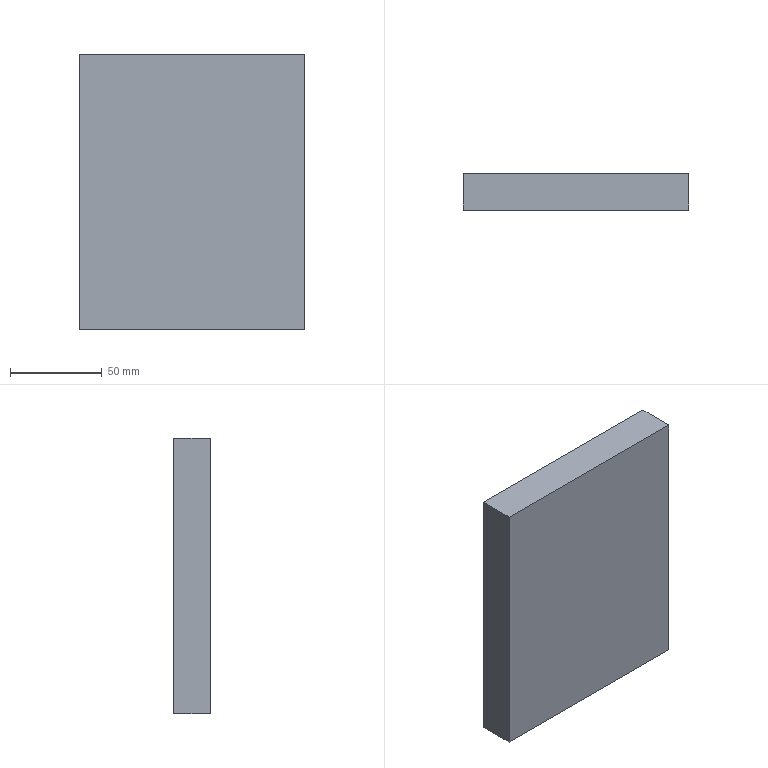Part | SolidWorks | features BaseBody 1 | 1 solid | 17 faces | box 123 x 20 x 150 mm | volume 56150 mm3 | plane 11 | cylinder 6 | commonest cylinder face diameters 5 x6
STEP:
#1=CARTESIAN_POINT('',(37.5,11.,-75.));
#2=VERTEX_POINT('',#1);
#3=CARTESIAN_POINT('',(42.5,11.,-75.));
#4=VERTEX_POINT('',#3);
#5=CARTESIAN_POINT('',(40.,11.,-75.));
#6=DIRECTION('',(0.,0.,1.));
#7=DIRECTION('',(1.,0.,0.));
#8=AXIS2_PLACEMENT_3D('',#5,#6,#7);
#9=CIRCLE('',#8,2.5);
#10=EDGE_CURVE('',#2,#4,#9,.T.);
#11=ORIENTED_EDGE('',*,*,#10,.F.);
#12=CARTESIAN_POINT('',(37.5,11.,-73.));
#13=VERTEX_POINT('',#12);
#14=CARTESIAN_POINT('',(37.5,11.,-75.));
#15=DIRECTION('',(0.,0.,1.));
#16=VECTOR('',#15,1000.);
#17=LINE('',#14,#16);
#18=EDGE_CURVE('',#2,#13,#17,.T.);
#19=ORIENTED_EDGE('',*,*,#18,.T.);
#20=CARTESIAN_POINT('',(42.5,11.,-73.));
#21=VERTEX_POINT('',#20);
#22=CARTESIAN_POINT('',(40.,11.,-73.));
#23=DIRECTION('',(0.,0.,1.));
#24=DIRECTION('',(1.,0.,0.));
#25=AXIS2_PLACEMENT_3D('',#22,#23,#24);
#26=CIRCLE('',#25,2.5);
#27=EDGE_CURVE('',#13,#21,#26,.T.);
#28=ORIENTED_EDGE('',*,*,#27,.T.);
#29=CARTESIAN_POINT('',(42.5,11.,-75.));
#30=DIRECTION('',(0.,0.,1.));
#31=VECTOR('',#30,1000.);
#32=LINE('',#29,#31);
#33=EDGE_CURVE('',#4,#21,#32,.T.);
#34=ORIENTED_EDGE('',*,*,#33,.F.);
#35=EDGE_LOOP('',(#11,#19,#28,#34));
#36=FACE_OUTER_BOUND('',#35,.T.);
#37=CARTESIAN_POINT('',(40.,11.,-75.));
#38=DIRECTION('',(0.,0.,1.));
#39=DIRECTION('',(1.,0.,0.));
#40=AXIS2_PLACEMENT_3D('',#37,#38,#39);
#41=CYLINDRICAL_SURFACE('',#40,2.5);
#42=ADVANCED_FACE('',(#36),#41,.F.);
#43=CARTESIAN_POINT('',(-2.5,11.,-75.));
#44=VERTEX_POINT('',#43);
#45=CARTESIAN_POINT('',(2.5,11.,-75.));
#46=VERTEX_POINT('',#45);
#47=CARTESIAN_POINT('',(0.,11.,-75.));
#48=DIRECTION('',(0.,0.,1.));
#49=DIRECTION('',(1.,0.,0.));
#50=AXIS2_PLACEMENT_3D('',#47,#48,#49);
#51=CIRCLE('',#50,2.5);
#52=EDGE_CURVE('',#44,#46,#51,.T.);
#53=ORIENTED_EDGE('',*,*,#52,.F.);
#54=CARTESIAN_POINT('',(-2.5,11.,-73.));
#55=VERTEX_POINT('',#54);
#56=CARTESIAN_POINT('',(-2.5,11.,-75.));
#57=DIRECTION('',(0.,0.,1.));
#58=VECTOR('',#57,1000.);
#59=LINE('',#56,#58);
#60=EDGE_CURVE('',#44,#55,#59,.T.);
#61=ORIENTED_EDGE('',*,*,#60,.T.);
#62=CARTESIAN_POINT('',(2.5,11.,-73.));
#63=VERTEX_POINT('',#62);
#64=CARTESIAN_POINT('',(0.,11.,-73.));
#65=DIRECTION('',(0.,0.,1.));
#66=DIRECTION('',(1.,0.,0.));
#67=AXIS2_PLACEMENT_3D('',#64,#65,#66);
#68=CIRCLE('',#67,2.5);
#69=EDGE_CURVE('',#55,#63,#68,.T.);
#70=ORIENTED_EDGE('',*,*,#69,.T.);
#71=CARTESIAN_POINT('',(2.5,11.,-75.));
#72=DIRECTION('',(0.,0.,1.));
#73=VECTOR('',#72,1000.);
#74=LINE('',#71,#73);
#75=EDGE_CURVE('',#46,#63,#74,.T.);
#76=ORIENTED_EDGE('',*,*,#75,.F.);
#77=EDGE_LOOP('',(#53,#61,#70,#76));
#78=FACE_OUTER_BOUND('',#77,.T.);
#79=CARTESIAN_POINT('',(0.,11.,-75.));
#80=DIRECTION('',(0.,0.,1.));
#81=DIRECTION('',(1.,0.,0.));
#82=AXIS2_PLACEMENT_3D('',#79,#80,#81);
#83=CYLINDRICAL_SURFACE('',#82,2.5);
#84=ADVANCED_FACE('',(#78),#83,.F.);
#85=CARTESIAN_POINT('',(-42.5,11.,-75.));
#86=VERTEX_POINT('',#85);
#87=CARTESIAN_POINT('',(-37.5,11.,-75.));
#88=VERTEX_POINT('',#87);
#89=CARTESIAN_POINT('',(-40.,11.,-75.));
#90=DIRECTION('',(0.,0.,1.));
#91=DIRECTION('',(1.,0.,0.));
#92=AXIS2_PLACEMENT_3D('',#89,#90,#91);
#93=CIRCLE('',#92,2.5);
#94=EDGE_CURVE('',#86,#88,#93,.T.);
#95=ORIENTED_EDGE('',*,*,#94,.F.);
#96=CARTESIAN_POINT('',(-42.5,11.,-73.));
#97=VERTEX_POINT('',#96);
#98=CARTESIAN_POINT('',(-42.5,11.,-75.));
#99=DIRECTION('',(0.,0.,1.));
#100=VECTOR('',#99,1000.);
#101=LINE('',#98,#100);
#102=EDGE_CURVE('',#86,#97,#101,.T.);
#103=ORIENTED_EDGE('',*,*,#102,.T.);
#104=CARTESIAN_POINT('',(-37.5,11.,-73.));
#105=VERTEX_POINT('',#104);
#106=CARTESIAN_POINT('',(-40.,11.,-73.));
#107=DIRECTION('',(0.,0.,1.));
#108=DIRECTION('',(1.,0.,0.));
#109=AXIS2_PLACEMENT_3D('',#106,#107,#108);
#110=CIRCLE('',#109,2.5);
#111=EDGE_CURVE('',#97,#105,#110,.T.);
#112=ORIENTED_EDGE('',*,*,#111,.T.);
#113=CARTESIAN_POINT('',(-37.5,11.,-75.));
#114=DIRECTION('',(0.,0.,1.));
#115=VECTOR('',#114,1000.);
#116=LINE('',#113,#115);
#117=EDGE_CURVE('',#88,#105,#116,.T.);
#118=ORIENTED_EDGE('',*,*,#117,.F.);
#119=EDGE_LOOP('',(#95,#103,#112,#118));
#120=FACE_OUTER_BOUND('',#119,.T.);
#121=CARTESIAN_POINT('',(-40.,11.,-75.));
#122=DIRECTION('',(0.,0.,1.));
#123=DIRECTION('',(1.,0.,0.));
#124=AXIS2_PLACEMENT_3D('',#121,#122,#123);
#125=CYLINDRICAL_SURFACE('',#124,2.5);
#126=ADVANCED_FACE('',(#120),#125,.F.);
#127=CARTESIAN_POINT('',(59.5,2.,73.));
#128=VERTEX_POINT('',#127);
#129=CARTESIAN_POINT('',(59.5,2.,-73.));
#130=VERTEX_POINT('',#129);
#131=CARTESIAN_POINT('',(59.5,2.,-75.));
#132=DIRECTION('',(0.,0.,-1.));
#133=VECTOR('',#132,1000.);
#134=LINE('',#131,#133);
#135=EDGE_CURVE('',#128,#130,#134,.T.);
#136=ORIENTED_EDGE('',*,*,#135,.T.);
#137=CARTESIAN_POINT('',(-59.5,2.,-73.));
#138=VERTEX_POINT('',#137);
#139=CARTESIAN_POINT('',(-61.5,2.,-73.));
#140=DIRECTION('',(-1.,0.,0.));
#141=VECTOR('',#140,1000.);
#142=LINE('',#139,#141);
#143=EDGE_CURVE('',#130,#138,#142,.T.);
#144=ORIENTED_EDGE('',*,*,#143,.T.);
#145=CARTESIAN_POINT('',(-59.5,2.,73.));
#146=VERTEX_POINT('',#145);
#147=CARTESIAN_POINT('',(-59.5,2.,-75.));
#148=DIRECTION('',(0.,0.,1.));
#149=VECTOR('',#148,1000.);
#150=LINE('',#147,#149);
#151=EDGE_CURVE('',#138,#146,#150,.T.);
#152=ORIENTED_EDGE('',*,*,#151,.T.);
#153=CARTESIAN_POINT('',(-61.5,2.,73.));
#154=DIRECTION('',(1.,0.,0.));
#155=VECTOR('',#154,1000.);
#156=LINE('',#153,#155);
#157=EDGE_CURVE('',#146,#128,#156,.T.);
#158=ORIENTED_EDGE('',*,*,#157,.T.);
#159=EDGE_LOOP('',(#136,#144,#152,#158));
#160=FACE_OUTER_BOUND('',#159,.T.);
#161=CARTESIAN_POINT('',(0.,2.,0.));
#162=DIRECTION('',(0.,1.,0.));
#163=DIRECTION('',(1.,0.,0.));
#164=AXIS2_PLACEMENT_3D('',#161,#162,#163);
#165=PLANE('',#164);
#166=ADVANCED_FACE('',(#160),#165,.T.);
#167=ORIENTED_EDGE('',*,*,#157,.F.);
#168=CARTESIAN_POINT('',(-59.5,20.,73.));
#169=VERTEX_POINT('',#168);
#170=CARTESIAN_POINT('',(-59.5,20.,73.));
#171=DIRECTION('',(0.,-1.,0.));
#172=VECTOR('',#171,1000.);
#173=LINE('',#170,#172);
#174=EDGE_CURVE('',#169,#146,#173,.T.);
#175=ORIENTED_EDGE('',*,*,#174,.F.);
#176=CARTESIAN_POINT('',(59.5,20.,73.));
#177=VERTEX_POINT('',#176);
#178=CARTESIAN_POINT('',(-61.5,20.,73.));
#179=DIRECTION('',(1.,0.,0.));
#180=VECTOR('',#179,1000.);
#181=LINE('',#178,#180);
#182=EDGE_CURVE('',#169,#177,#181,.T.);
#183=ORIENTED_EDGE('',*,*,#182,.T.);
#184=CARTESIAN_POINT('',(59.5,20.,73.));
#185=DIRECTION('',(0.,-1.,0.));
#186=VECTOR('',#185,1000.);
#187=LINE('',#184,#186);
#188=EDGE_CURVE('',#177,#128,#187,.T.);
#189=ORIENTED_EDGE('',*,*,#188,.T.);
#190=EDGE_LOOP('',(#167,#175,#183,#189));
#191=FACE_OUTER_BOUND('',#190,.T.);
#192=CARTESIAN_POINT('',(-61.5,20.,73.));
#193=DIRECTION('',(0.,0.,-1.));
#194=DIRECTION('',(0.,-1.,0.));
#195=AXIS2_PLACEMENT_3D('',#192,#193,#194);
#196=PLANE('',#195);
#197=ADVANCED_FACE('',(#191),#196,.T.);
#198=ORIENTED_EDGE('',*,*,#151,.F.);
#199=CARTESIAN_POINT('',(-59.5,20.,-73.));
#200=VERTEX_POINT('',#199);
#201=CARTESIAN_POINT('',(-59.5,20.,-73.));
#202=DIRECTION('',(0.,-1.,0.));
#203=VECTOR('',#202,1000.);
#204=LINE('',#201,#203);
#205=EDGE_CURVE('',#200,#138,#204,.T.);
#206=ORIENTED_EDGE('',*,*,#205,.F.);
#207=CARTESIAN_POINT('',(-59.5,20.,-75.));
#208=DIRECTION('',(0.,0.,1.));
#209=VECTOR('',#208,1000.);
#210=LINE('',#207,#209);
#211=EDGE_CURVE('',#200,#169,#210,.T.);
#212=ORIENTED_EDGE('',*,*,#211,.T.);
#213=ORIENTED_EDGE('',*,*,#174,.T.);
#214=EDGE_LOOP('',(#198,#206,#212,#213));
#215=FACE_OUTER_BOUND('',#214,.T.);
#216=CARTESIAN_POINT('',(-59.5,20.,-75.));
#217=DIRECTION('',(1.,0.,0.));
#218=DIRECTION('',(0.,0.,-1.));
#219=AXIS2_PLACEMENT_3D('',#216,#217,#218);
#220=PLANE('',#219);
#221=ADVANCED_FACE('',(#215),#220,.T.);
#222=CARTESIAN_POINT('',(-40.,11.,-73.));
#223=DIRECTION('',(0.,0.,1.));
#224=DIRECTION('',(1.,0.,0.));
#225=AXIS2_PLACEMENT_3D('',#222,#223,#224);
#226=CIRCLE('',#225,2.5);
#227=EDGE_CURVE('',#105,#97,#226,.T.);
#228=ORIENTED_EDGE('',*,*,#227,.F.);
#229=ORIENTED_EDGE('',*,*,#111,.F.);
#230=EDGE_LOOP('',(#228,#229));
#231=FACE_BOUND('',#230,.T.);
#232=CARTESIAN_POINT('',(0.,11.,-73.));
#233=DIRECTION('',(0.,0.,1.));
#234=DIRECTION('',(1.,0.,0.));
#235=AXIS2_PLACEMENT_3D('',#232,#233,#234);
#236=CIRCLE('',#235,2.5);
#237=EDGE_CURVE('',#63,#55,#236,.T.);
#238=ORIENTED_EDGE('',*,*,#237,.F.);
#239=ORIENTED_EDGE('',*,*,#69,.F.);
#240=EDGE_LOOP('',(#238,#239));
#241=FACE_BOUND('',#240,.T.);
#242=CARTESIAN_POINT('',(40.,11.,-73.));
#243=DIRECTION('',(0.,0.,1.));
#244=DIRECTION('',(1.,0.,0.));
#245=AXIS2_PLACEMENT_3D('',#242,#243,#244);
#246=CIRCLE('',#245,2.5);
#247=EDGE_CURVE('',#21,#13,#246,.T.);
#248=ORIENTED_EDGE('',*,*,#247,.F.);
#249=ORIENTED_EDGE('',*,*,#27,.F.);
#250=EDGE_LOOP('',(#248,#249));
#251=FACE_BOUND('',#250,.T.);
#252=ORIENTED_EDGE('',*,*,#143,.F.);
#253=CARTESIAN_POINT('',(59.5,20.,-73.));
#254=VERTEX_POINT('',#253);
#255=CARTESIAN_POINT('',(59.5,20.,-73.));
#256=DIRECTION('',(0.,-1.,0.));
#257=VECTOR('',#256,1000.);
#258=LINE('',#255,#257);
#259=EDGE_CURVE('',#254,#130,#258,.T.);
#260=ORIENTED_EDGE('',*,*,#259,.F.);
#261=CARTESIAN_POINT('',(-61.5,20.,-73.));
#262=DIRECTION('',(-1.,0.,0.));
#263=VECTOR('',#262,1000.);
#264=LINE('',#261,#263);
#265=EDGE_CURVE('',#254,#200,#264,.T.);
#266=ORIENTED_EDGE('',*,*,#265,.T.);
#267=ORIENTED_EDGE('',*,*,#205,.T.);
#268=EDGE_LOOP('',(#252,#260,#266,#267));
#269=FACE_OUTER_BOUND('',#268,.T.);
#270=CARTESIAN_POINT('',(-61.5,20.,-73.));
#271=DIRECTION('',(0.,0.,1.));
#272=DIRECTION('',(1.,0.,0.));
#273=AXIS2_PLACEMENT_3D('',#270,#271,#272);
#274=PLANE('',#273);
#275=ADVANCED_FACE('',(#231,#241,#251,#269),#274,.T.);
#276=ORIENTED_EDGE('',*,*,#135,.F.);
#277=ORIENTED_EDGE('',*,*,#188,.F.);
#278=CARTESIAN_POINT('',(59.5,20.,-75.));
#279=DIRECTION('',(0.,0.,-1.));
#280=VECTOR('',#279,1000.);
#281=LINE('',#278,#280);
#282=EDGE_CURVE('',#177,#254,#281,.T.);
#283=ORIENTED_EDGE('',*,*,#282,.T.);
#284=ORIENTED_EDGE('',*,*,#259,.T.);
#285=EDGE_LOOP('',(#276,#277,#283,#284));
#286=FACE_OUTER_BOUND('',#285,.T.);
#287=CARTESIAN_POINT('',(59.5,20.,-75.));
#288=DIRECTION('',(-1.,0.,0.));
#289=DIRECTION('',(0.,1.,0.));
#290=AXIS2_PLACEMENT_3D('',#287,#288,#289);
#291=PLANE('',#290);
#292=ADVANCED_FACE('',(#286),#291,.T.);
#293=CARTESIAN_POINT('',(61.5,0.,75.));
#294=VERTEX_POINT('',#293);
#295=CARTESIAN_POINT('',(61.5,0.,-75.));
#296=VERTEX_POINT('',#295);
#297=CARTESIAN_POINT('',(61.5,0.,-75.));
#298=DIRECTION('',(0.,0.,-1.));
#299=VECTOR('',#298,1000.);
#300=LINE('',#297,#299);
#301=EDGE_CURVE('',#294,#296,#300,.T.);
#302=ORIENTED_EDGE('',*,*,#301,.F.);
#303=CARTESIAN_POINT('',(-61.5,0.,75.));
#304=VERTEX_POINT('',#303);
#305=CARTESIAN_POINT('',(-61.5,0.,75.));
#306=DIRECTION('',(1.,0.,0.));
#307=VECTOR('',#306,1000.);
#308=LINE('',#305,#307);
#309=EDGE_CURVE('',#304,#294,#308,.T.);
#310=ORIENTED_EDGE('',*,*,#309,.F.);
#311=CARTESIAN_POINT('',(-61.5,0.,-75.));
#312=VERTEX_POINT('',#311);
#313=CARTESIAN_POINT('',(-61.5,0.,-75.));
#314=DIRECTION('',(0.,0.,1.));
#315=VECTOR('',#314,1000.);
#316=LINE('',#313,#315);
#317=EDGE_CURVE('',#312,#304,#316,.T.);
#318=ORIENTED_EDGE('',*,*,#317,.F.);
#319=CARTESIAN_POINT('',(-61.5,0.,-75.));
#320=DIRECTION('',(-1.,0.,0.));
#321=VECTOR('',#320,1000.);
#322=LINE('',#319,#321);
#323=EDGE_CURVE('',#296,#312,#322,.T.);
#324=ORIENTED_EDGE('',*,*,#323,.F.);
#325=EDGE_LOOP('',(#302,#310,#318,#324));
#326=FACE_OUTER_BOUND('',#325,.T.);
#327=CARTESIAN_POINT('',(0.,0.,0.));
#328=DIRECTION('',(0.,1.,0.));
#329=DIRECTION('',(1.,0.,0.));
#330=AXIS2_PLACEMENT_3D('',#327,#328,#329);
#331=PLANE('',#330);
#332=ADVANCED_FACE('',(#326),#331,.F.);
#333=ORIENTED_EDGE('',*,*,#282,.F.);
#334=ORIENTED_EDGE('',*,*,#182,.F.);
#335=ORIENTED_EDGE('',*,*,#211,.F.);
#336=ORIENTED_EDGE('',*,*,#265,.F.);
#337=EDGE_LOOP('',(#333,#334,#335,#336));
#338=FACE_BOUND('',#337,.T.);
#339=CARTESIAN_POINT('',(61.5,20.,75.));
#340=VERTEX_POINT('',#339);
#341=CARTESIAN_POINT('',(61.5,20.,-75.));
#342=VERTEX_POINT('',#341);
#343=CARTESIAN_POINT('',(61.5,20.,-75.));
#344=DIRECTION('',(0.,0.,-1.));
#345=VECTOR('',#344,1000.);
#346=LINE('',#343,#345);
#347=EDGE_CURVE('',#340,#342,#346,.T.);
#348=ORIENTED_EDGE('',*,*,#347,.T.);
#349=CARTESIAN_POINT('',(-61.5,20.,-75.));
#350=VERTEX_POINT('',#349);
#351=CARTESIAN_POINT('',(-61.5,20.,-75.));
#352=DIRECTION('',(-1.,0.,0.));
#353=VECTOR('',#352,1000.);
#354=LINE('',#351,#353);
#355=EDGE_CURVE('',#342,#350,#354,.T.);
#356=ORIENTED_EDGE('',*,*,#355,.T.);
#357=CARTESIAN_POINT('',(-61.5,20.,75.));
#358=VERTEX_POINT('',#357);
#359=CARTESIAN_POINT('',(-61.5,20.,-75.));
#360=DIRECTION('',(0.,0.,1.));
#361=VECTOR('',#360,1000.);
#362=LINE('',#359,#361);
#363=EDGE_CURVE('',#350,#358,#362,.T.);
#364=ORIENTED_EDGE('',*,*,#363,.T.);
#365=CARTESIAN_POINT('',(-61.5,20.,75.));
#366=DIRECTION('',(1.,0.,0.));
#367=VECTOR('',#366,1000.);
#368=LINE('',#365,#367);
#369=EDGE_CURVE('',#358,#340,#368,.T.);
#370=ORIENTED_EDGE('',*,*,#369,.T.);
#371=EDGE_LOOP('',(#348,#356,#364,#370));
#372=FACE_OUTER_BOUND('',#371,.T.);
#373=CARTESIAN_POINT('',(0.,20.,0.));
#374=DIRECTION('',(0.,1.,0.));
#375=DIRECTION('',(1.,0.,0.));
#376=AXIS2_PLACEMENT_3D('',#373,#374,#375);
#377=PLANE('',#376);
#378=ADVANCED_FACE('',(#338,#372),#377,.T.);
#379=ORIENTED_EDGE('',*,*,#309,.T.);
#380=CARTESIAN_POINT('',(61.5,20.,75.));
#381=DIRECTION('',(0.,-1.,0.));
#382=VECTOR('',#381,1000.);
#383=LINE('',#380,#382);
#384=EDGE_CURVE('',#340,#294,#383,.T.);
#385=ORIENTED_EDGE('',*,*,#384,.F.);
#386=ORIENTED_EDGE('',*,*,#369,.F.);
#387=CARTESIAN_POINT('',(-61.5,20.,75.));
#388=DIRECTION('',(0.,-1.,0.));
#389=VECTOR('',#388,1000.);
#390=LINE('',#387,#389);
#391=EDGE_CURVE('',#358,#304,#390,.T.);
#392=ORIENTED_EDGE('',*,*,#391,.T.);
#393=EDGE_LOOP('',(#379,#385,#386,#392));
#394=FACE_OUTER_BOUND('',#393,.T.);
#395=CARTESIAN_POINT('',(-61.5,20.,75.));
#396=DIRECTION('',(0.,0.,-1.));
#397=DIRECTION('',(0.,-1.,0.));
#398=AXIS2_PLACEMENT_3D('',#395,#396,#397);
#399=PLANE('',#398);
#400=ADVANCED_FACE('',(#394),#399,.F.);
#401=ORIENTED_EDGE('',*,*,#317,.T.);
#402=ORIENTED_EDGE('',*,*,#391,.F.);
#403=ORIENTED_EDGE('',*,*,#363,.F.);
#404=CARTESIAN_POINT('',(-61.5,20.,-75.));
#405=DIRECTION('',(0.,-1.,0.));
#406=VECTOR('',#405,1000.);
#407=LINE('',#404,#406);
#408=EDGE_CURVE('',#350,#312,#407,.T.);
#409=ORIENTED_EDGE('',*,*,#408,.T.);
#410=EDGE_LOOP('',(#401,#402,#403,#409));
#411=FACE_OUTER_BOUND('',#410,.T.);
#412=CARTESIAN_POINT('',(-61.5,20.,-75.));
#413=DIRECTION('',(1.,0.,0.));
#414=DIRECTION('',(0.,0.,-1.));
#415=AXIS2_PLACEMENT_3D('',#412,#413,#414);
#416=PLANE('',#415);
#417=ADVANCED_FACE('',(#411),#416,.F.);
#418=CARTESIAN_POINT('',(-40.,11.,-75.));
#419=DIRECTION('',(0.,0.,1.));
#420=DIRECTION('',(1.,0.,0.));
#421=AXIS2_PLACEMENT_3D('',#418,#419,#420);
#422=CIRCLE('',#421,2.5);
#423=EDGE_CURVE('',#88,#86,#422,.T.);
#424=ORIENTED_EDGE('',*,*,#423,.T.);
#425=ORIENTED_EDGE('',*,*,#94,.T.);
#426=EDGE_LOOP('',(#424,#425));
#427=FACE_BOUND('',#426,.T.);
#428=CARTESIAN_POINT('',(0.,11.,-75.));
#429=DIRECTION('',(0.,0.,1.));
#430=DIRECTION('',(1.,0.,0.));
#431=AXIS2_PLACEMENT_3D('',#428,#429,#430);
#432=CIRCLE('',#431,2.5);
#433=EDGE_CURVE('',#46,#44,#432,.T.);
#434=ORIENTED_EDGE('',*,*,#433,.T.);
#435=ORIENTED_EDGE('',*,*,#52,.T.);
#436=EDGE_LOOP('',(#434,#435));
#437=FACE_BOUND('',#436,.T.);
#438=CARTESIAN_POINT('',(40.,11.,-75.));
#439=DIRECTION('',(0.,0.,1.));
#440=DIRECTION('',(1.,0.,0.));
#441=AXIS2_PLACEMENT_3D('',#438,#439,#440);
#442=CIRCLE('',#441,2.5);
#443=EDGE_CURVE('',#4,#2,#442,.T.);
#444=ORIENTED_EDGE('',*,*,#443,.T.);
#445=ORIENTED_EDGE('',*,*,#10,.T.);
#446=EDGE_LOOP('',(#444,#445));
#447=FACE_BOUND('',#446,.T.);
#448=ORIENTED_EDGE('',*,*,#323,.T.);
#449=ORIENTED_EDGE('',*,*,#408,.F.);
#450=ORIENTED_EDGE('',*,*,#355,.F.);
#451=CARTESIAN_POINT('',(61.5,20.,-75.));
#452=DIRECTION('',(0.,-1.,0.));
#453=VECTOR('',#452,1000.);
#454=LINE('',#451,#453);
#455=EDGE_CURVE('',#342,#296,#454,.T.);
#456=ORIENTED_EDGE('',*,*,#455,.T.);
#457=EDGE_LOOP('',(#448,#449,#450,#456));
#458=FACE_OUTER_BOUND('',#457,.T.);
#459=CARTESIAN_POINT('',(-61.5,20.,-75.));
#460=DIRECTION('',(0.,0.,1.));
#461=DIRECTION('',(1.,0.,0.));
#462=AXIS2_PLACEMENT_3D('',#459,#460,#461);
#463=PLANE('',#462);
#464=ADVANCED_FACE('',(#427,#437,#447,#458),#463,.F.);
#465=ORIENTED_EDGE('',*,*,#301,.T.);
#466=ORIENTED_EDGE('',*,*,#455,.F.);
#467=ORIENTED_EDGE('',*,*,#347,.F.);
#468=ORIENTED_EDGE('',*,*,#384,.T.);
#469=EDGE_LOOP('',(#465,#466,#467,#468));
#470=FACE_OUTER_BOUND('',#469,.T.);
#471=CARTESIAN_POINT('',(61.5,20.,-75.));
#472=DIRECTION('',(-1.,0.,0.));
#473=DIRECTION('',(0.,1.,0.));
#474=AXIS2_PLACEMENT_3D('',#471,#472,#473);
#475=PLANE('',#474);
#476=ADVANCED_FACE('',(#470),#475,.F.);
#477=ORIENTED_EDGE('',*,*,#102,.F.);
#478=ORIENTED_EDGE('',*,*,#423,.F.);
#479=ORIENTED_EDGE('',*,*,#117,.T.);
#480=ORIENTED_EDGE('',*,*,#227,.T.);
#481=EDGE_LOOP('',(#477,#478,#479,#480));
#482=FACE_OUTER_BOUND('',#481,.T.);
#483=CARTESIAN_POINT('',(-40.,11.,-75.));
#484=DIRECTION('',(0.,0.,1.));
#485=DIRECTION('',(1.,0.,0.));
#486=AXIS2_PLACEMENT_3D('',#483,#484,#485);
#487=CYLINDRICAL_SURFACE('',#486,2.5);
#488=ADVANCED_FACE('',(#482),#487,.F.);
#489=ORIENTED_EDGE('',*,*,#60,.F.);
#490=ORIENTED_EDGE('',*,*,#433,.F.);
#491=ORIENTED_EDGE('',*,*,#75,.T.);
#492=ORIENTED_EDGE('',*,*,#237,.T.);
#493=EDGE_LOOP('',(#489,#490,#491,#492));
#494=FACE_OUTER_BOUND('',#493,.T.);
#495=CARTESIAN_POINT('',(0.,11.,-75.));
#496=DIRECTION('',(0.,0.,1.));
#497=DIRECTION('',(1.,0.,0.));
#498=AXIS2_PLACEMENT_3D('',#495,#496,#497);
#499=CYLINDRICAL_SURFACE('',#498,2.5);
#500=ADVANCED_FACE('',(#494),#499,.F.);
#501=ORIENTED_EDGE('',*,*,#18,.F.);
#502=ORIENTED_EDGE('',*,*,#443,.F.);
#503=ORIENTED_EDGE('',*,*,#33,.T.);
#504=ORIENTED_EDGE('',*,*,#247,.T.);
#505=EDGE_LOOP('',(#501,#502,#503,#504));
#506=FACE_OUTER_BOUND('',#505,.T.);
#507=CARTESIAN_POINT('',(40.,11.,-75.));
#508=DIRECTION('',(0.,0.,1.));
#509=DIRECTION('',(1.,0.,0.));
#510=AXIS2_PLACEMENT_3D('',#507,#508,#509);
#511=CYLINDRICAL_SURFACE('',#510,2.5);
#512=ADVANCED_FACE('',(#506),#511,.F.);
#513=CLOSED_SHELL('',(#42,#84,#126,#166,#197,#221,#275,#292,#332,#378,#400,#417,#464,#476,#488,#500,#512));
#514=MANIFOLD_SOLID_BREP('',#513);
#515=CARTESIAN_POINT('',(0.,0.,0.));
#516=DIRECTION('',(0.,0.,1.));
#517=DIRECTION('',(1.,0.,0.));
#518=AXIS2_PLACEMENT_3D('',#515,#516,#517);
#519=(LENGTH_UNIT()NAMED_UNIT(*)SI_UNIT(.MILLI.,.METRE.));
#520=UNCERTAINTY_MEASURE_WITH_UNIT(LENGTH_MEASURE(0.00001),#519,'','');
#521=(NAMED_UNIT(*)PLANE_ANGLE_UNIT()SI_UNIT($,.RADIAN.));
#522=(NAMED_UNIT(*)SI_UNIT($,.STERADIAN.)SOLID_ANGLE_UNIT());
#523=(GEOMETRIC_REPRESENTATION_CONTEXT(3)GLOBAL_UNCERTAINTY_ASSIGNED_CONTEXT((#520))GLOBAL_UNIT_ASSIGNED_CONTEXT((#519,#521,#522))REPRESENTATION_CONTEXT('',''));
#524=ADVANCED_BREP_SHAPE_REPRESENTATION('',(#514,#518),#523);